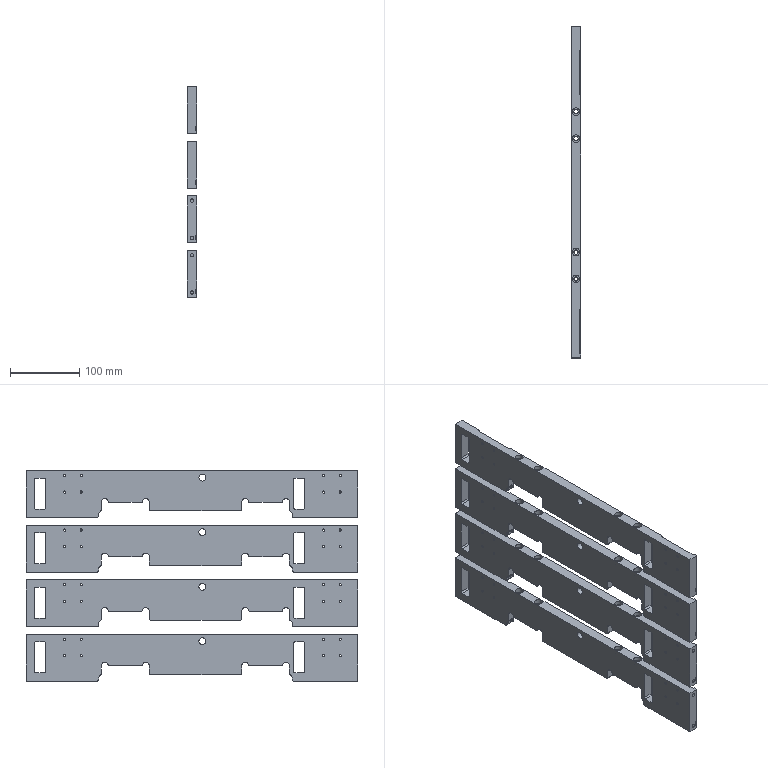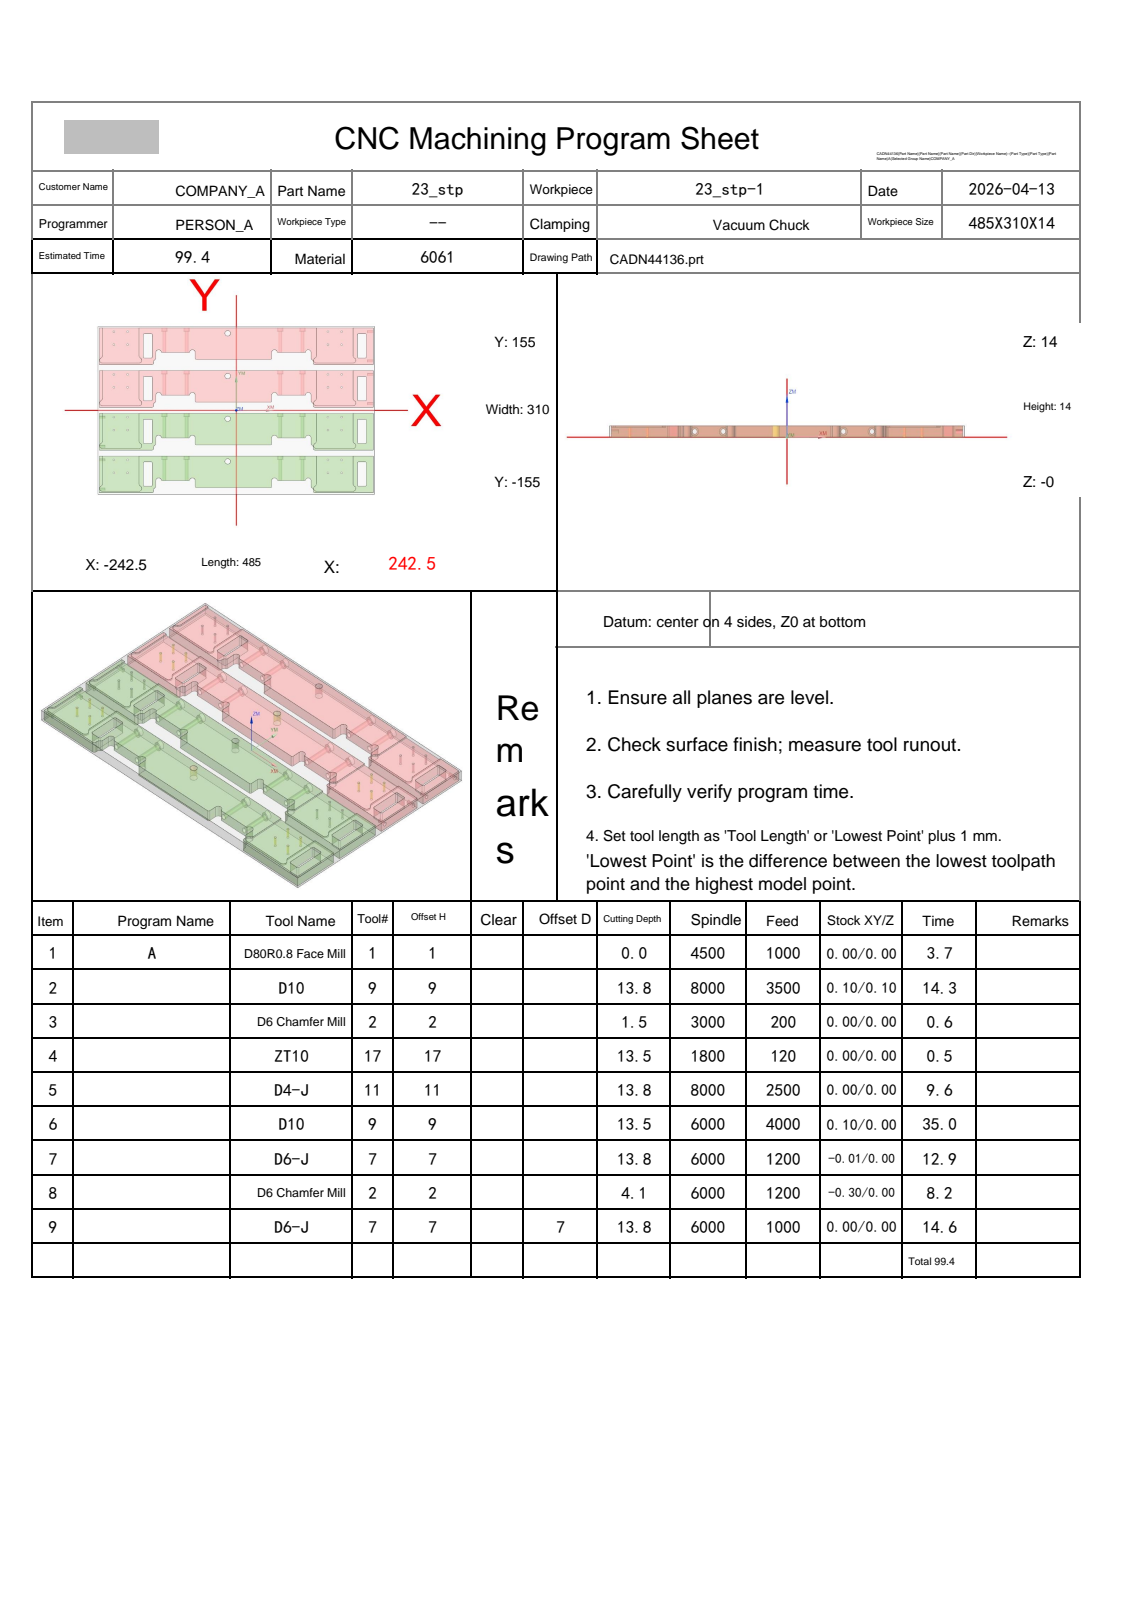NC program | NX | posted by the shop | part box 14 x 480 x 305 mm
Lines 2633 to 3570 of 51894:
N5 T11 M06
(D4-J  D=4. R=0. H=11 ce=0.00 di=0.01)
G00 G90 G54 X-160.399 Y-134.684 M03 S6000
G43 H11 Z34.
M08
Z14.3
G01 X-160.406 Y-134.685 Z14.214 F2000.
X-160.425 Y-134.688 Z14.136
X-160.455 Y-134.694 Z14.066
X-160.493 Y-134.703 Z14.004
X-160.538 Y-134.715 Z13.948
X-160.589 Y-134.73 Z13.899
X-160.644 Y-134.748 Z13.857
X-160.7 Y-134.77 Z13.82
X-160.756 Y-134.796 Z13.789
X-160.81 Y-134.826 Z13.763
X-160.861 Y-134.859 Z13.742
X-160.906 Y-134.897 Z13.726
X-160.945 Y-134.94 Z13.714
X-160.974 Y-134.987 Z13.706
X-160.993 Y-135.04 Z13.701
X-161. Y-135.097 Z13.7
Y-138.25 F2500.
X-157.847
X-157.804 Y-138.234 Z13.699
X-157.782 Y-138.188 Z13.696
X-157.781 Y-138.115 Z13.692
X-157.798 Y-138.02 Z13.687
X-157.831 Y-137.905 Z13.68
X-157.88 Y-137.773 Z13.672
X-157.943 Y-137.629 Z13.662
X-158.017 Y-137.475 Z13.653
X-158.102 Y-137.316 Z13.642
X-158.196 Y-137.154 Z13.631
X-158.296 Y-136.993 Z13.619
X-158.538 Y-136.653 Z13.592
X-158.805 Y-136.336 Z13.564
X-159.097 Y-136.042 Z13.536
X-159.412 Y-135.775 Z13.508
X-159.75 Y-135.534 Z13.481
X-159.91 Y-135.434 Z13.469
X-160.071 Y-135.342 Z13.458
X-160.229 Y-135.258 Z13.447
X-160.382 Y-135.185 Z13.438
X-160.525 Y-135.124 Z13.428
X-160.656 Y-135.077 Z13.42
X-160.771 Y-135.045 Z13.413
X-160.866 Y-135.029 Z13.408
X-160.938 Y-135.031 Z13.404
X-160.984 Y-135.054 Z13.401
X-161. Y-135.097 Z13.4
Y-138.25
X-157.847
X-157.804 Y-138.234 Z13.399
X-157.782 Y-138.188 Z13.398
X-157.781 Y-138.115 Z13.395
X-157.798 Y-138.019 Z13.392
X-157.832 Y-137.904 Z13.388
X-157.881 Y-137.772 Z13.383
X-157.943 Y-137.627 Z13.378
X-158.018 Y-137.473 Z13.372
X-158.103 Y-137.313 Z13.366
X-158.197 Y-137.151 Z13.359
X-158.298 Y-136.989 Z13.352
X-158.54 Y-136.648 Z13.336
X-158.807 Y-136.33 Z13.318
X-159.099 Y-136.036 Z13.296
X-159.415 Y-135.768 Z13.271
X-159.752 Y-135.528 Z13.24
X-159.912 Y-135.428 Z13.224
X-160.073 Y-135.337 Z13.207
X-160.231 Y-135.254 Z13.19
X-160.384 Y-135.181 Z13.173
X-160.527 Y-135.121 Z13.157
X-160.657 Y-135.075 Z13.141
X-160.771 Y-135.043 Z13.128
X-160.866 Y-135.028 Z13.116
X-160.938 Y-135.031 Z13.108
X-160.984 Y-135.053 Z13.102
X-161. Y-135.097 Z13.1
Y-138.25
X-157.847
X-157.804 Y-138.234 Z13.099
X-157.782 Y-138.188 Z13.098
X-157.781 Y-138.115 Z13.095
X-157.798 Y-138.019 Z13.092
X-157.832 Y-137.903 Z13.088
X-157.881 Y-137.771 Z13.083
X-157.944 Y-137.626 Z13.078
X-158.018 Y-137.471 Z13.072
X-158.151 Y-137.227 Z13.062
X-158.298 Y-136.986 Z13.052
X-158.54 Y-136.643 Z13.036
X-158.808 Y-136.324 Z13.018
X-159.1 Y-136.029 Z12.996
X-159.415 Y-135.761 Z12.971
X-159.753 Y-135.521 Z12.94
X-159.912 Y-135.422 Z12.924
X-160.073 Y-135.331 Z12.907
X-160.231 Y-135.249 Z12.89
X-160.384 Y-135.177 Z12.873
X-160.527 Y-135.118 Z12.857
X-160.657 Y-135.072 Z12.841
X-160.772 Y-135.041 Z12.828
X-160.866 Y-135.027 Z12.816
X-160.938 Y-135.03 Z12.808
X-160.984 Y-135.053 Z12.802
X-161. Y-135.097 Z12.8
Y-138.25
X-157.847
X-157.804 Y-138.234 Z12.799
X-157.782 Y-138.187 Z12.798
X-157.781 Y-138.114 Z12.795
X-157.798 Y-138.018 Z12.792
X-157.832 Y-137.902 Z12.788
X-157.881 Y-137.769 Z12.783
X-157.944 Y-137.624 Z12.778
X-158.018 Y-137.469 Z12.772
X-158.152 Y-137.224 Z12.762
X-158.298 Y-136.982 Z12.752
X-158.54 Y-136.638 Z12.736
X-158.808 Y-136.318 Z12.717
X-159.1 Y-136.022 Z12.696
X-159.416 Y-135.754 Z12.671
X-159.753 Y-135.514 Z12.64
X-159.913 Y-135.416 Z12.624
X-160.073 Y-135.325 Z12.607
X-160.232 Y-135.244 Z12.59
X-160.384 Y-135.173 Z12.573
X-160.527 Y-135.115 Z12.556
X-160.657 Y-135.07 Z12.541
X-160.772 Y-135.04 Z12.528
X-160.866 Y-135.026 Z12.516
X-160.938 Y-135.03 Z12.508
X-160.984 Y-135.053 Z12.502
X-161. Y-135.097 Z12.5
Y-138.25
X-157.847
X-157.804 Y-138.234 Z12.499
X-157.782 Y-138.187 Z12.498
X-157.781 Y-138.114 Z12.495
X-157.798 Y-138.017 Z12.492
X-157.832 Y-137.901 Z12.488
X-157.881 Y-137.768 Z12.483
X-157.944 Y-137.622 Z12.478
X-158.019 Y-137.467 Z12.472
X-158.152 Y-137.221 Z12.462
X-158.299 Y-136.978 Z12.452
X-158.541 Y-136.633 Z12.436
X-158.809 Y-136.311 Z12.417
X-159.101 Y-136.015 Z12.396
X-159.416 Y-135.746 Z12.37
X-159.754 Y-135.507 Z12.34
X-159.913 Y-135.409 Z12.324
X-160.074 Y-135.319 Z12.307
X-160.232 Y-135.239 Z12.29
X-160.384 Y-135.169 Z12.273
X-160.527 Y-135.111 Z12.256
X-160.658 Y-135.067 Z12.241
X-160.772 Y-135.038 Z12.228
X-160.867 Y-135.025 Z12.216
X-160.938 Y-135.03 Z12.208
X-160.984 Y-135.053 Z12.202
X-161. Y-135.097 Z12.2
Y-138.25
X-157.847
X-157.804 Y-138.234 Z12.199
X-157.782 Y-138.187 Z12.198
X-157.781 Y-138.114 Z12.195
X-157.798 Y-138.017 Z12.192
X-157.832 Y-137.9 Z12.188
X-157.881 Y-137.767 Z12.183
X-157.944 Y-137.62 Z12.178
X-158.019 Y-137.464 Z12.172
X-158.152 Y-137.218 Z12.162
X-158.299 Y-136.974 Z12.152
X-158.541 Y-136.628 Z12.135
X-158.809 Y-136.305 Z12.117
X-159.102 Y-136.008 Z12.096
X-159.417 Y-135.739 Z12.07
X-159.754 Y-135.5 Z12.039
X-159.914 Y-135.403 Z12.023
X-160.075 Y-135.314 Z12.007
X-160.233 Y-135.234 Z11.99
X-160.385 Y-135.165 Z11.973
X-160.528 Y-135.108 Z11.956
X-160.658 Y-135.065 Z11.941
X-160.772 Y-135.036 Z11.928
X-160.867 Y-135.024 Z11.916
X-160.938 Y-135.029 Z11.908
X-160.984 Y-135.053 Z11.902
X-161. Y-135.097 Z11.9
Y-138.25
X-157.847
X-157.804 Y-138.234 Z11.899
X-157.782 Y-138.187 Z11.898
X-157.781 Y-138.113 Z11.895
X-157.798 Y-138.016 Z11.892
X-157.832 Y-137.899 Z11.888
X-157.881 Y-137.765 Z11.883
X-157.944 Y-137.618 Z11.878
X-158.019 Y-137.462 Z11.872
X-158.153 Y-137.215 Z11.862
X-158.3 Y-136.97 Z11.851
X-158.542 Y-136.622 Z11.835
X-158.81 Y-136.298 Z11.817
X-159.103 Y-136. Z11.795
X-159.418 Y-135.731 Z11.77
X-159.755 Y-135.493 Z11.739
X-159.915 Y-135.396 Z11.723
X-160.075 Y-135.308 Z11.706
X-160.233 Y-135.229 Z11.689
X-160.385 Y-135.161 Z11.672
X-160.528 Y-135.105 Z11.656
X-160.658 Y-135.062 Z11.641
X-160.772 Y-135.035 Z11.628
X-160.867 Y-135.023 Z11.616
X-160.939 Y-135.029 Z11.608
X-160.984 Y-135.053 Z11.602
X-161. Y-135.097 Z11.6
Y-138.25
X-157.847
X-157.804 Y-138.234 Z11.599
X-157.782 Y-138.187 Z11.598
X-157.781 Y-138.113 Z11.595
X-157.798 Y-138.015 Z11.592
X-157.832 Y-137.898 Z11.588
X-157.882 Y-137.764 Z11.583
X-157.945 Y-137.616 Z11.578
X-158.019 Y-137.46 Z11.572
X-158.153 Y-137.211 Z11.562
X-158.3 Y-136.966 Z11.551
X-158.543 Y-136.617 Z11.535
X-158.811 Y-136.292 Z11.517
X-159.104 Y-135.993 Z11.495
X-159.419 Y-135.723 Z11.47
X-159.756 Y-135.486 Z11.439
X-159.916 Y-135.389 Z11.423
X-160.076 Y-135.301 Z11.406
X-160.234 Y-135.223 Z11.389
X-160.386 Y-135.156 Z11.372
X-160.529 Y-135.101 Z11.356
X-160.659 Y-135.06 Z11.341
X-160.772 Y-135.033 Z11.328
X-160.867 Y-135.022 Z11.316
X-160.939 Y-135.028 Z11.308
X-160.984 Y-135.053 Z11.302
X-161. Y-135.097 Z11.3
Y-138.25
X-157.847
X-157.804 Y-138.234 Z11.299
X-157.782 Y-138.187 Z11.298
X-157.781 Y-138.112 Z11.295
X-157.798 Y-138.015 Z11.292
X-157.832 Y-137.897 Z11.288
X-157.882 Y-137.762 Z11.283
X-157.945 Y-137.614 Z11.277
X-158.02 Y-137.457 Z11.271
X-158.154 Y-137.208 Z11.261
X-158.301 Y-136.962 Z11.251
X-158.544 Y-136.611 Z11.235
X-158.812 Y-136.285 Z11.216
X-159.105 Y-135.985 Z11.195
X-159.42 Y-135.715 Z11.169
X-159.758 Y-135.478 Z11.138
X-159.917 Y-135.382 Z11.123
X-160.077 Y-135.295 Z11.106
X-160.235 Y-135.218 Z11.089
X-160.387 Y-135.152 Z11.072
X-160.529 Y-135.098 Z11.056
X-160.659 Y-135.057 Z11.041
X-160.773 Y-135.031 Z11.027
X-160.867 Y-135.021 Z11.016
X-160.939 Y-135.028 Z11.008
X-160.984 Y-135.053 Z11.002
X-161. Y-135.097 Z11.
Y-138.25
X-157.847
X-157.804 Y-138.234 Z10.999
X-157.782 Y-138.186 Z10.998
X-157.781 Y-138.112 Z10.995
X-157.799 Y-138.014 Z10.992
X-157.833 Y-137.896 Z10.988
X-157.882 Y-137.761 Z10.983
X-157.945 Y-137.613 Z10.977
X-158.02 Y-137.455 Z10.971
X-158.154 Y-137.205 Z10.961
X-158.302 Y-136.957 Z10.951
X-158.545 Y-136.606 Z10.934
X-158.814 Y-136.278 Z10.916
X-159.106 Y-135.977 Z10.894
X-159.422 Y-135.707 Z10.869
X-159.759 Y-135.471 Z10.838
X-159.918 Y-135.376 Z10.822
X-160.078 Y-135.289 Z10.806
X-160.236 Y-135.213 Z10.789
X-160.388 Y-135.147 Z10.772
X-160.53 Y-135.094 Z10.756
X-160.66 Y-135.054 Z10.741
X-160.773 Y-135.029 Z10.727
X-160.867 Y-135.02 Z10.716
X-160.939 Y-135.027 Z10.707
X-160.984 Y-135.052 Z10.702
X-161. Y-135.097 Z10.7
Y-138.25
X-157.847
X-157.804 Y-138.233 Z10.699
X-157.783 Y-138.186 Z10.698
X-157.781 Y-138.112 Z10.695
X-157.799 Y-138.013 Z10.692
X-157.833 Y-137.895 Z10.688
X-157.882 Y-137.759 Z10.683
X-157.946 Y-137.611 Z10.677
X-158.021 Y-137.452 Z10.671
X-158.155 Y-137.201 Z10.661
X-158.303 Y-136.953 Z10.651
X-158.546 Y-136.6 Z10.634
X-158.815 Y-136.271 Z10.615
X-159.108 Y-135.97 Z10.594
X-159.424 Y-135.699 Z10.568
X-159.761 Y-135.463 Z10.538
X-159.92 Y-135.368 Z10.522
X-160.08 Y-135.283 Z10.505
X-160.237 Y-135.207 Z10.488
X-160.389 Y-135.143 Z10.472
X-160.531 Y-135.09 Z10.455
X-160.66 Y-135.051 Z10.441
X-160.774 Y-135.027 Z10.427
X-160.868 Y-135.018 Z10.416
X-160.939 Y-135.026 Z10.407
X-160.984 Y-135.052 Z10.402
X-161. Y-135.097 Z10.4
Y-138.25
X-157.847
X-157.804 Y-138.233 Z10.399
X-157.783 Y-138.186 Z10.398
X-157.781 Y-138.111 Z10.395
X-157.799 Y-138.012 Z10.392
X-157.833 Y-137.894 Z10.388
X-157.883 Y-137.758 Z10.383
X-157.946 Y-137.609 Z10.377
X-158.022 Y-137.45 Z10.371
X-158.156 Y-137.198 Z10.361
X-158.304 Y-136.949 Z10.35
X-158.548 Y-136.594 Z10.334
X-158.817 Y-136.264 Z10.315
X-159.11 Y-135.962 Z10.293
X-159.426 Y-135.691 Z10.268
X-159.763 Y-135.455 Z10.237
X-159.922 Y-135.361 Z10.221
X-160.081 Y-135.276 Z10.205
X-160.239 Y-135.201 Z10.188
X-160.39 Y-135.138 Z10.171
X-160.532 Y-135.087 Z10.155
X-160.661 Y-135.049 Z10.14
X-160.774 Y-135.025 Z10.127
X-160.868 Y-135.017 Z10.116
X-160.939 Y-135.026 Z10.107
X-160.984 Y-135.052 Z10.102
X-161. Y-135.097 Z10.1
Y-138.25
X-157.847
X-157.804 Y-138.233 Z10.099
X-157.783 Y-138.186 Z10.098
X-157.782 Y-138.111 Z10.095
X-157.799 Y-138.012 Z10.092
X-157.834 Y-137.892 Z10.088
X-157.883 Y-137.756 Z10.083
X-157.947 Y-137.606 Z10.077
X-158.022 Y-137.447 Z10.071
X-158.157 Y-137.195 Z10.061
X-158.305 Y-136.944 Z10.05
X-158.549 Y-136.589 Z10.033
X-158.819 Y-136.257 Z10.014
X-159.112 Y-135.954 Z9.993
X-159.428 Y-135.683 Z9.967
X-159.765 Y-135.448 Z9.937
X-159.924 Y-135.354 Z9.921
X-160.083 Y-135.27 Z9.904
X-160.24 Y-135.196 Z9.887
X-160.391 Y-135.133 Z9.871
X-160.533 Y-135.083 Z9.855
X-160.662 Y-135.046 Z9.84
X-160.775 Y-135.023 Z9.827
X-160.868 Y-135.016 Z9.816
X-160.939 Y-135.025 Z9.807
X-160.984 Y-135.052 Z9.802
X-161. Y-135.097 Z9.8
Y-138.25
X-157.847
X-157.804 Y-138.233 Z9.799
X-157.783 Y-138.186 Z9.798
X-157.782 Y-138.11 Z9.795
X-157.799 Y-138.011 Z9.792
X-157.834 Y-137.891 Z9.787
X-157.884 Y-137.755 Z9.782
X-157.947 Y-137.604 Z9.777
X-158.023 Y-137.444 Z9.771
X-158.158 Y-137.191 Z9.76
X-158.306 Y-136.94 Z9.75
X-158.551 Y-136.583 Z9.733
X-158.821 Y-136.25 Z9.714
X-159.115 Y-135.946 Z9.692
X-159.431 Y-135.674 Z9.667
X-159.767 Y-135.44 Z9.636
X-159.926 Y-135.347 Z9.62
X-160.085 Y-135.263 Z9.604
X-160.242 Y-135.19 Z9.587
X-160.393 Y-135.128 Z9.57
X-160.534 Y-135.079 Z9.555
X-160.662 Y-135.043 Z9.54
X-160.775 Y-135.021 Z9.527
X-160.869 Y-135.015 Z9.516
X-160.939 Y-135.025 Z9.507
X-160.984 Y-135.052 Z9.502
X-161. Y-135.097 Z9.5
Y-138.25
X-157.847
X-157.804 Y-138.233 Z9.499
X-157.783 Y-138.185 Z9.498
X-157.782 Y-138.11 Z9.495
X-157.8 Y-138.01 Z9.492
X-157.834 Y-137.89 Z9.487
X-157.884 Y-137.753 Z9.482
X-157.948 Y-137.602 Z9.477
X-158.024 Y-137.442 Z9.47
X-158.159 Y-137.187 Z9.46
X-158.308 Y-136.935 Z9.449
X-158.553 Y-136.577 Z9.432
X-158.823 Y-136.243 Z9.413
X-159.118 Y-135.937 Z9.391
X-159.434 Y-135.666 Z9.366
X-159.77 Y-135.432 Z9.335
X-159.928 Y-135.339 Z9.32
X-160.088 Y-135.257 Z9.303
X-160.244 Y-135.184 Z9.287
X-160.394 Y-135.124 Z9.27
X-160.535 Y-135.075 Z9.254
X-160.663 Y-135.04 Z9.24
X-160.776 Y-135.019 Z9.227
X-160.869 Y-135.014 Z9.216
X-160.94 Y-135.024 Z9.207
X-160.984 Y-135.052 Z9.202
X-161. Y-135.097 Z9.2
Y-138.25
X-157.847
X-157.804 Y-138.233 Z9.199
X-157.783 Y-138.185 Z9.198
X-157.782 Y-138.109 Z9.195
X-157.8 Y-138.01 Z9.192
X-157.835 Y-137.889 Z9.187
X-157.885 Y-137.751 Z9.182
X-157.949 Y-137.6 Z9.176
X-158.025 Y-137.439 Z9.17
X-158.16 Y-137.184 Z9.16
X-158.31 Y-136.931 Z9.149
X-158.555 Y-136.571 Z9.132
X-158.826 Y-136.235 Z9.113
X-159.121 Y-135.929 Z9.091
X-159.437 Y-135.657 Z9.065
X-159.773 Y-135.424 Z9.034
X-159.931 Y-135.332 Z9.019
X-160.09 Y-135.25 Z9.003
X-160.246 Y-135.179 Z8.986
X-160.396 Y-135.119 Z8.97
X-160.537 Y-135.071 Z8.954
X-160.664 Y-135.037 Z8.939
X-160.777 Y-135.018 Z8.926
X-160.869 Y-135.013 Z8.916
X-160.94 Y-135.024 Z8.907
X-160.984 Y-135.052 Z8.902
X-161. Y-135.097 Z8.9
Y-138.25
X-157.847
X-157.804 Y-138.233 Z8.899
X-157.783 Y-138.185 Z8.898
X-157.782 Y-138.109 Z8.895
X-157.8 Y-138.009 Z8.892
X-157.835 Y-137.888 Z8.887
X-157.886 Y-137.75 Z8.882
X-157.95 Y-137.598 Z8.876
X-158.026 Y-137.436 Z8.87
X-158.162 Y-137.18 Z8.859
X-158.311 Y-136.926 Z8.848
X-158.558 Y-136.565 Z8.831
X-158.829 Y-136.228 Z8.812
X-159.124 Y-135.921 Z8.79
X-159.44 Y-135.649 Z8.764
X-159.776 Y-135.416 Z8.734
X-159.934 Y-135.325 Z8.718
X-160.093 Y-135.243 Z8.702
X-160.248 Y-135.173 Z8.685
X-160.398 Y-135.114 Z8.669
X-160.538 Y-135.068 Z8.654
X-160.666 Y-135.035 Z8.639
X-160.777 Y-135.016 Z8.626
X-160.87 Y-135.012 Z8.615
X-160.94 Y-135.023 Z8.607
X-160.984 Y-135.051 Z8.602
X-161. Y-135.097 Z8.6
Y-138.25
X-157.847
X-157.804 Y-138.233 Z8.599
X-157.783 Y-138.185 Z8.598
X-157.782 Y-138.109 Z8.595
X-157.8 Y-138.008 Z8.591
X-157.836 Y-137.887 Z8.587
X-157.886 Y-137.748 Z8.582
X-157.951 Y-137.596 Z8.576
X-158.027 Y-137.434 Z8.57
X-158.163 Y-137.177 Z8.559
X-158.313 Y-136.922 Z8.548
X-158.517 Y-136.618 Z8.533
X-158.739 Y-136.33 Z8.518
X-158.977 Y-136.063 Z8.5
X-159.231 Y-135.818 Z8.481
X-159.499 Y-135.598 Z8.458
X-159.78 Y-135.408 Z8.433
X-159.937 Y-135.317 Z8.417
X-160.096 Y-135.237 Z8.401
X-160.251 Y-135.167 Z8.385
X-160.4 Y-135.109 Z8.369
X-160.54 Y-135.064 Z8.353
X-160.667 Y-135.032 Z8.339
X-160.778 Y-135.014 Z8.326
X-160.87 Y-135.01 Z8.315
X-160.94 Y-135.023 Z8.307
X-160.985 Y-135.051 Z8.302
X-161. Y-135.097 Z8.3
Y-138.25
X-157.847
X-157.804 Y-138.233 Z8.299
X-157.783 Y-138.185 Z8.298
Y-138.108 Z8.295
X-157.801 Y-138.007 Z8.291
X-157.836 Y-137.886 Z8.287
X-157.887 Y-137.747 Z8.282
X-157.952 Y-137.594 Z8.276
X-158.028 Y-137.431 Z8.269
X-158.165 Y-137.173 Z8.259
X-158.316 Y-136.917 Z8.247
X-158.52 Y-136.612 Z8.233
X-158.742 Y-136.323 Z8.217
X-158.981 Y-136.055 Z8.199
X-159.235 Y-135.809 Z8.18
X-159.503 Y-135.59 Z8.157
X-159.784 Y-135.4 Z8.132
X-159.941 Y-135.31 Z8.116
X-160.099 Y-135.23 Z8.1
X-160.254 Y-135.161 Z8.084
X-160.402 Y-135.104 Z8.068
X-160.542 Y-135.06 Z8.053
X-160.668 Y-135.029 Z8.038
X-160.779 Y-135.012 Z8.026
X-160.871 Y-135.009 Z8.015
X-160.941 Y-135.022 Z8.007
X-160.985 Y-135.051 Z8.002
X-161. Y-135.097 Z8.
Y-138.25
X-157.847
X-157.804 Y-138.233 Z7.999
X-157.783 Y-138.184 Z7.998
Y-138.108 Z7.995
X-157.801 Y-138.007 Z7.991
X-157.837 Y-137.885 Z7.987
X-157.888 Y-137.745 Z7.981
X-157.953 Y-137.592 Z7.975
X-158.03 Y-137.429 Z7.969
X-158.167 Y-137.17 Z7.958
X-158.318 Y-136.913 Z7.947
X-158.523 Y-136.606 Z7.932
X-158.746 Y-136.316 Z7.916
X-158.985 Y-136.047 Z7.898
X-159.239 Y-135.801 Z7.879
X-159.507 Y-135.581 Z7.856
X-159.788 Y-135.392 Z7.831
X-159.961 Y-135.294 Z7.814
X-160.134 Y-135.209 Z7.796
X-160.302 Y-135.137 Z7.779
X-160.462 Y-135.081 Z7.761
X-160.609 Y-135.039 Z7.745
X-160.738 Y-135.014 Z7.73
X-160.846 Y-135.007 Z7.718
X-160.929 Y-135.018 Z7.708
X-160.982 Y-135.047 Z7.702
X-161. Y-135.097 Z7.7
Y-138.25
X-157.847
X-157.804 Y-138.233 Z7.699
X-157.783 Y-138.184 Z7.698
Y-138.107 Z7.695
X-157.802 Y-138.006 Z7.691
X-157.837 Y-137.883 Z7.687
X-157.889 Y-137.744 Z7.681
X-157.954 Y-137.59 Z7.675
X-158.031 Y-137.426 Z7.669
X-158.169 Y-137.166 Z7.658
X-158.321 Y-136.908 Z7.646
X-158.526 Y-136.6 Z7.631
X-158.75 Y-136.31 Z7.615
X-158.99 Y-136.039 Z7.597
X-159.244 Y-135.792 Z7.578
X-159.512 Y-135.573 Z7.555
X-159.792 Y-135.384 Z7.53
X-159.965 Y-135.287 Z7.513
X-160.137 Y-135.202 Z7.495
X-160.305 Y-135.132 Z7.478
X-160.464 Y-135.076 Z7.461
X-160.61 Y-135.036 Z7.445
X-160.739 Y-135.012 Z7.43
X-160.847 Y-135.006 Z7.418
X-160.929 Y-135.017 Z7.408
X-160.982 Y-135.047 Z7.402
X-161. Y-135.097 Z7.4
Y-138.25
X-157.847
X-157.804 Y-138.233 Z7.399
X-157.783 Y-138.184 Z7.398
Y-138.107 Z7.395
X-157.802 Y-138.005 Z7.391
X-157.838 Y-137.882 Z7.386
X-157.89 Y-137.742 Z7.381
X-157.955 Y-137.588 Z7.375
X-158.079 Y-137.334 Z7.364
X-158.171 Y-137.163 Z7.357
X-158.323 Y-136.904 Z7.345
X-158.53 Y-136.595 Z7.33
X-158.754 Y-136.303 Z7.314
X-158.994 Y-136.031 Z7.296
X-159.249 Y-135.784 Z7.276
X-159.517 Y-135.564 Z7.254
X-159.797 Y-135.376 Z7.229
X-159.969 Y-135.279 Z7.212
X-160.141 Y-135.196 Z7.194
X-160.309 Y-135.126 Z7.177
X-160.467 Y-135.072 Z7.16
X-160.612 Y-135.033 Z7.144
X-160.741 Y-135.01 Z7.13
X-160.848 Y-135.004 Z7.118
X-160.93 Y-135.016 Z7.108
X-160.982 Y-135.047 Z7.102
X-161. Y-135.097 Z7.1
Y-138.25
X-157.847
X-157.804 Y-138.233 Z7.099
X-157.784 Y-138.184 Z7.098
Y-138.106 Z7.095
X-157.803 Y-138.004 Z7.091
X-157.839 Y-137.881 Z7.086
X-157.891 Y-137.74 Z7.081
X-157.957 Y-137.586 Z7.075
X-158.081 Y-137.331 Z7.064
X-158.174 Y-137.159 Z7.057
X-158.326 Y-136.899 Z7.045
X-158.534 Y-136.589 Z7.029
X-158.759 Y-136.296 Z7.013
X-158.999 Y-136.024 Z6.995
X-159.255 Y-135.776 Z6.975
X-159.523 Y-135.556 Z6.953
X-159.802 Y-135.368 Z6.927
X-159.974 Y-135.272 Z6.911
X-160.146 Y-135.189 Z6.893
X-160.312 Y-135.121 Z6.876
X-160.47 Y-135.067 Z6.859
X-160.615 Y-135.029 Z6.843
X-160.742 Y-135.008 Z6.829
X-160.849 Y-135.003 Z6.817
X-160.93 Y-135.016 Z6.808
X-160.982 Y-135.047 Z6.802
X-161. Y-135.097 Z6.8
Y-138.25
X-157.847
X-157.804 Y-138.233 Z6.799
X-157.784 Y-138.184 Z6.798
Y-138.106 Z6.795
X-157.803 Y-138.004 Z6.791
X-157.84 Y-137.88 Z6.786
X-157.892 Y-137.739 Z6.78
X-157.958 Y-137.584 Z6.774
X-158.083 Y-137.328 Z6.763
X-158.176 Y-137.156 Z6.756
X-158.329 Y-136.895 Z6.744
X-158.538 Y-136.584 Z6.729
X-158.763 Y-136.289 Z6.712
X-159.005 Y-136.016 Z6.694
X-159.261 Y-135.768 Z6.674
X-159.529 Y-135.548 Z6.651
X-159.808 Y-135.36 Z6.626
X-159.979 Y-135.265 Z6.609
X-160.15 Y-135.183 Z6.592
X-160.316 Y-135.116 Z6.575
X-160.473 Y-135.063 Z6.559
X-160.617 Y-135.026 Z6.543
X-160.744 Y-135.005 Z6.529
X-160.85 Y-135.001 Z6.517
X-160.931 Y-135.015 Z6.508
X-160.982 Y-135.047 Z6.502
X-161. Y-135.097 Z6.5
Y-138.25
X-157.847
X-157.804 Y-138.233 Z6.499
X-157.784 Y-138.183 Z6.498
Y-138.106 Z6.495
X-157.804 Y-138.003 Z6.491
X-157.84 Y-137.879 Z6.486
X-157.893 Y-137.737 Z6.48
X-157.96 Y-137.582 Z6.474
X-158.085 Y-137.325 Z6.463
X-158.179 Y-137.152 Z6.455
X-158.333 Y-136.891 Z6.443
X-158.542 Y-136.578 Z6.428
X-158.769 Y-136.283 Z6.411
X-159.011 Y-136.009 Z6.392
X-159.267 Y-135.76 Z6.372
X-159.535 Y-135.54 Z6.35
X-159.814 Y-135.353 Z6.325
X-159.985 Y-135.258 Z6.308
X-160.155 Y-135.177 Z6.291
X-160.32 Y-135.11 Z6.274
X-160.476 Y-135.059 Z6.258
X-160.619 Y-135.023 Z6.242
X-160.746 Y-135.003 Z6.229
X-160.851 Y-135. Z6.217
X-160.931 Y-135.014 Z6.208
X-160.982 Y-135.046 Z6.202
X-161. Y-135.097 Z6.2
Y-138.25
X-157.847
X-157.804 Y-138.233 Z6.199
X-157.784 Y-138.183 Z6.197
X-157.785 Y-138.105 Z6.195
X-157.804 Y-138.002 Z6.191
X-157.841 Y-137.878 Z6.186
X-157.894 Y-137.736 Z6.18
X-157.961 Y-137.58 Z6.173
X-158.088 Y-137.322 Z6.162
X-158.182 Y-137.149 Z6.155
X-158.336 Y-136.886 Z6.142
X-158.546 Y-136.573 Z6.126
X-158.774 Y-136.276 Z6.109
X-159.017 Y-136.001 Z6.091
X-159.273 Y-135.752 Z6.071
X-159.542 Y-135.532 Z6.048
X-159.82 Y-135.345 Z6.023
X-159.991 Y-135.251 Z6.007
X-160.16 Y-135.171 Z5.99
X-160.324 Y-135.105 Z5.973
X-160.48 Y-135.055 Z5.957
X-160.622 Y-135.02 Z5.942
X-160.748 Y-135.001 Z5.928
X-160.852 Y-134.999 Z5.917
X-160.932 Y-135.014 Z5.908
X-160.982 Y-135.046 Z5.902
X-161. Y-135.097 Z5.9
Y-138.25
X-157.847
X-157.804 Y-138.233 Z5.899
X-157.784 Y-138.183 Z5.897
X-157.785 Y-138.105 Z5.894
X-157.805 Y-138.002 Z5.89
X-157.842 Y-137.877 Z5.885
X-157.896 Y-137.734 Z5.88
X-157.963 Y-137.578 Z5.873
X-158.09 Y-137.32 Z5.862
X-158.184 Y-137.146 Z5.854
X-158.34 Y-136.882 Z5.842
X-158.551 Y-136.567 Z5.825
X-158.78 Y-136.27 Z5.808
X-159.023 Y-135.994 Z5.789
X-159.28 Y-135.744 Z5.769
X-159.549 Y-135.524 Z5.747
X-159.827 Y-135.338 Z5.722
X-159.997 Y-135.244 Z5.705
X-160.165 Y-135.165 Z5.689
X-160.329 Y-135.1 Z5.672
X-160.483 Y-135.051 Z5.656
X-160.625 Y-135.017 Z5.641
X-160.749 Y-134.999 Z5.628
X-160.853 Y-134.997 Z5.616
X-160.932 Y-135.013 Z5.608
X-160.982 Y-135.046 Z5.602
X-161. Y-135.097 Z5.6
Y-138.25
X-157.847
X-157.804 Y-138.233 Z5.599
X-157.784 Y-138.183 Z5.597
X-157.785 Y-138.104 Z5.594
X-157.805 Y-138.001 Z5.59
X-157.843 Y-137.876 Z5.585
X-157.897 Y-137.733 Z5.579
X-157.965 Y-137.576 Z5.573
X-158.093 Y-137.317 Z5.561
X-158.188 Y-137.142 Z5.553
X-158.344 Y-136.878 Z5.541
X-158.556 Y-136.562 Z5.524
X-158.786 Y-136.264 Z5.507
X-159.03 Y-135.987 Z5.488
X-159.288 Y-135.737 Z5.467
X-159.556 Y-135.516 Z5.445
X-159.834 Y-135.331 Z5.42
X-160.003 Y-135.238 Z5.404
X-160.171 Y-135.159 Z5.387
X-160.334 Y-135.095 Z5.371
X-160.487 Y-135.047 Z5.355
X-160.628 Y-135.014 Z5.34
X-160.751 Y-134.997 Z5.327
X-160.854 Y-134.996 Z5.316
X-160.933 Y-135.012 Z5.307
X-160.983 Y-135.046 Z5.302
X-161. Y-135.097 Z5.3
Y-138.25
X-157.847
X-157.804 Y-138.233 Z5.299
X-157.785 Y-138.183 Z5.297
X-157.786 Y-138.104 Z5.294
X-157.806 Y-138. Z5.29
X-157.844 Y-137.875 Z5.285
X-157.898 Y-137.732 Z5.279
X-157.967 Y-137.574 Z5.272
X-158.095 Y-137.314 Z5.261
X-158.191 Y-137.139 Z5.252
X-158.348 Y-136.874 Z5.24
X-158.562 Y-136.557 Z5.223
X-158.792 Y-136.258 Z5.205
X-159.037 Y-135.98 Z5.186
X-159.295 Y-135.729 Z5.166
X-159.564 Y-135.509 Z5.143
X-159.841 Y-135.324 Z5.118
X-160.01 Y-135.231 Z5.102
X-160.177 Y-135.153 Z5.086
X-160.339 Y-135.091 Z5.07
X-160.491 Y-135.043 Z5.054
X-160.631 Y-135.011 Z5.04
X-160.754 Y-134.995 Z5.027
X-160.856 Z5.016
X-160.933 Y-135.012 Z5.007
X-160.983 Y-135.046 Z5.002
X-161. Y-135.097 Z5.
Y-138.25
X-157.847
X-157.804 Y-138.233 Z4.999
X-157.785 Y-138.183 Z4.997
X-157.786 Y-138.104 Z4.994
X-157.807 Y-138. Z4.99
X-157.845 Y-137.874 Z4.985
X-157.9 Y-137.73 Z4.979
X-157.969 Y-137.572 Z4.972
X-158.098 Y-137.312 Z4.96
X-158.194 Y-137.136 Z4.952
X-158.352 Y-136.87 Z4.939
X-158.567 Y-136.552 Z4.922
X-158.799 Y-136.252 Z4.904
X-159.045 Y-135.974 Z4.884
X-159.304 Y-135.722 Z4.864
X-159.572 Y-135.502 Z4.841
X-159.849 Y-135.317 Z4.816
X-160.017 Y-135.225 Z4.801
X-160.183 Y-135.148 Z4.785
X-160.344 Y-135.086 Z4.769
X-160.496 Y-135.039 Z4.753
X-160.634 Y-135.008 Z4.739
X-160.756 Y-134.993 Z4.726
X-160.857 Y-134.994 Z4.715
X-160.934 Y-135.011 Z4.707
X-160.983 Y-135.046 Z4.702
X-161. Y-135.097 Z4.7
Y-138.25
X-157.847
X-157.807 Y-138.235 Z4.699
X-157.787 Y-138.193 Z4.698
X-157.784 Y-138.126 Z4.695
X-157.799 Y-138.036 Z4.691
X-157.828 Y-137.928 Z4.687
X-157.872 Y-137.803 Z4.681
X-157.929 Y-137.665 Z4.675
X-158.038 Y-137.432 Z4.665
X-158.176 Y-137.174 Z4.653
X-158.357 Y-136.867 Z4.638
X-158.573 Y-136.548 Z4.62
X-158.806 Y-136.247 Z4.602
X-159.053 Y-135.968 Z4.583
X-159.312 Y-135.715 Z4.562
X-159.581 Y-135.495 Z4.539
X-159.857 Y-135.311 Z4.515
X-160.024 Y-135.219 Z4.499
X-160.19 Y-135.143 Z4.483
X-160.35 Y-135.081 Z4.467
X-160.5 Y-135.036 Z4.452
X-160.637 Y-135.005 Z4.438
X-160.758 Y-134.991 Z4.426
X-160.858 Y-134.993 Z4.415
X-160.935 Y-135.011 Z4.407
X-160.983 Y-135.045 Z4.402
X-161. Y-135.097 Z4.4
Y-138.25
X-157.847
X-157.807 Y-138.235 Z4.399
X-157.787 Y-138.193 Z4.398
X-157.785 Y-138.125 Z4.395
X-157.799 Y-138.036 Z4.391
X-157.829 Y-137.927 Z4.387
X-157.874 Y-137.802 Z4.381
X-157.931 Y-137.663 Z4.375
X-158.041 Y-137.43 Z4.364
X-158.179 Y-137.171 Z4.352
X-158.362 Y-136.863 Z4.337
X-158.579 Y-136.543 Z4.319
X-158.813 Y-136.241 Z4.3
X-159.061 Y-135.962 Z4.281
X-159.321 Y-135.709 Z4.26
X-159.59 Y-135.488 Z4.237
X-159.865 Y-135.305 Z4.213
X-160.032 Y-135.214 Z4.197
X-160.197 Y-135.138 Z4.182
X-160.355 Y-135.077 Z4.166
X-160.505 Y-135.032 Z4.151
X-160.641 Y-135.003 Z4.137
X-160.761 Y-134.989 Z4.125
X-160.86 Y-134.992 Z4.115
X-160.935 Y-135.01 Z4.107
X-160.983 Y-135.045 Z4.102
X-161. Y-135.097 Z4.1
Y-138.25
X-157.847
X-157.807 Y-138.235 Z4.099
X-157.787 Y-138.193 Z4.098
X-157.785 Y-138.125 Z4.095
X-157.8 Y-138.035 Z4.091
X-157.83 Y-137.927 Z4.086
X-157.875 Y-137.801 Z4.081
X-157.932 Y-137.662 Z4.074
X-158.044 Y-137.428 Z4.064
X-158.183 Y-137.169 Z4.051
X-158.367 Y-136.86 Z4.035
X-158.585 Y-136.539 Z4.018
X-158.82 Y-136.236 Z3.999
X-159.069 Y-135.956 Z3.979
X-159.33 Y-135.703 Z3.958